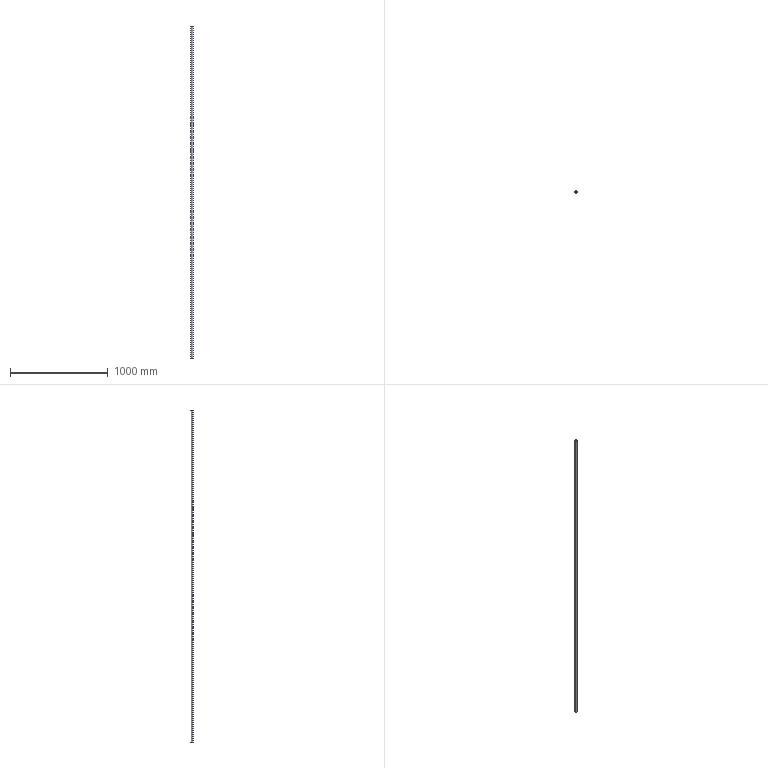Part | SolidWorks | features Extrusion 1 | 1 solid | 6 faces | box 25 x 25 x 3400 mm | volume 491345 mm3 | cylinder 4 | plane 2 | commonest cylinder face diameters 21 x2 25 x2
STEP:
#1=CARTESIAN_POINT('',(-10.5,0.,1700.));
#2=VERTEX_POINT('',#1);
#3=CARTESIAN_POINT('',(10.5,0.,1700.));
#4=VERTEX_POINT('',#3);
#5=CARTESIAN_POINT('',(0.,0.,1700.));
#6=DIRECTION('',(0.,0.,1.));
#7=DIRECTION('',(1.,0.,0.));
#8=AXIS2_PLACEMENT_3D('',#5,#6,#7);
#9=CIRCLE('',#8,10.5);
#10=EDGE_CURVE('',#2,#4,#9,.T.);
#11=ORIENTED_EDGE('',*,*,#10,.T.);
#12=CARTESIAN_POINT('',(10.5,0.,-1700.));
#13=VERTEX_POINT('',#12);
#14=CARTESIAN_POINT('',(10.5,0.,1700.));
#15=DIRECTION('',(0.,0.,-1.));
#16=VECTOR('',#15,1000.);
#17=LINE('',#14,#16);
#18=EDGE_CURVE('',#4,#13,#17,.T.);
#19=ORIENTED_EDGE('',*,*,#18,.T.);
#20=CARTESIAN_POINT('',(-10.5,0.,-1700.));
#21=VERTEX_POINT('',#20);
#22=CARTESIAN_POINT('',(0.,0.,-1700.));
#23=DIRECTION('',(0.,0.,1.));
#24=DIRECTION('',(1.,0.,0.));
#25=AXIS2_PLACEMENT_3D('',#22,#23,#24);
#26=CIRCLE('',#25,10.5);
#27=EDGE_CURVE('',#21,#13,#26,.T.);
#28=ORIENTED_EDGE('',*,*,#27,.F.);
#29=CARTESIAN_POINT('',(-10.5,0.,1700.));
#30=DIRECTION('',(0.,0.,-1.));
#31=VECTOR('',#30,1000.);
#32=LINE('',#29,#31);
#33=EDGE_CURVE('',#2,#21,#32,.T.);
#34=ORIENTED_EDGE('',*,*,#33,.F.);
#35=EDGE_LOOP('',(#11,#19,#28,#34));
#36=FACE_OUTER_BOUND('',#35,.T.);
#37=CARTESIAN_POINT('',(0.,0.,1700.));
#38=DIRECTION('',(0.,0.,-1.));
#39=DIRECTION('',(-1.,0.,0.));
#40=AXIS2_PLACEMENT_3D('',#37,#38,#39);
#41=CYLINDRICAL_SURFACE('',#40,10.5);
#42=ADVANCED_FACE('',(#36),#41,.F.);
#43=CARTESIAN_POINT('',(12.5,0.,1700.));
#44=VERTEX_POINT('',#43);
#45=CARTESIAN_POINT('',(-12.5,0.,1700.));
#46=VERTEX_POINT('',#45);
#47=CARTESIAN_POINT('',(0.,0.,1700.));
#48=DIRECTION('',(0.,0.,1.));
#49=DIRECTION('',(1.,0.,0.));
#50=AXIS2_PLACEMENT_3D('',#47,#48,#49);
#51=CIRCLE('',#50,12.5);
#52=EDGE_CURVE('',#44,#46,#51,.T.);
#53=ORIENTED_EDGE('',*,*,#52,.F.);
#54=CARTESIAN_POINT('',(12.5,0.,-1700.));
#55=VERTEX_POINT('',#54);
#56=CARTESIAN_POINT('',(12.5,0.,1700.));
#57=DIRECTION('',(0.,0.,-1.));
#58=VECTOR('',#57,1000.);
#59=LINE('',#56,#58);
#60=EDGE_CURVE('',#44,#55,#59,.T.);
#61=ORIENTED_EDGE('',*,*,#60,.T.);
#62=CARTESIAN_POINT('',(-12.5,0.,-1700.));
#63=VERTEX_POINT('',#62);
#64=CARTESIAN_POINT('',(0.,0.,-1700.));
#65=DIRECTION('',(0.,0.,1.));
#66=DIRECTION('',(1.,0.,0.));
#67=AXIS2_PLACEMENT_3D('',#64,#65,#66);
#68=CIRCLE('',#67,12.5);
#69=EDGE_CURVE('',#55,#63,#68,.T.);
#70=ORIENTED_EDGE('',*,*,#69,.T.);
#71=CARTESIAN_POINT('',(-12.5,0.,1700.));
#72=DIRECTION('',(0.,0.,-1.));
#73=VECTOR('',#72,1000.);
#74=LINE('',#71,#73);
#75=EDGE_CURVE('',#46,#63,#74,.T.);
#76=ORIENTED_EDGE('',*,*,#75,.F.);
#77=EDGE_LOOP('',(#53,#61,#70,#76));
#78=FACE_OUTER_BOUND('',#77,.T.);
#79=CARTESIAN_POINT('',(0.,0.,1700.));
#80=DIRECTION('',(0.,0.,-1.));
#81=DIRECTION('',(-1.,0.,0.));
#82=AXIS2_PLACEMENT_3D('',#79,#80,#81);
#83=CYLINDRICAL_SURFACE('',#82,12.5);
#84=ADVANCED_FACE('',(#78),#83,.T.);
#85=CARTESIAN_POINT('',(0.,0.,1700.));
#86=DIRECTION('',(0.,0.,1.));
#87=DIRECTION('',(1.,0.,0.));
#88=AXIS2_PLACEMENT_3D('',#85,#86,#87);
#89=CIRCLE('',#88,12.5);
#90=EDGE_CURVE('',#46,#44,#89,.T.);
#91=ORIENTED_EDGE('',*,*,#90,.T.);
#92=ORIENTED_EDGE('',*,*,#52,.T.);
#93=EDGE_LOOP('',(#91,#92));
#94=FACE_OUTER_BOUND('',#93,.T.);
#95=ORIENTED_EDGE('',*,*,#10,.F.);
#96=CARTESIAN_POINT('',(0.,0.,1700.));
#97=DIRECTION('',(0.,0.,1.));
#98=DIRECTION('',(1.,0.,0.));
#99=AXIS2_PLACEMENT_3D('',#96,#97,#98);
#100=CIRCLE('',#99,10.5);
#101=EDGE_CURVE('',#4,#2,#100,.T.);
#102=ORIENTED_EDGE('',*,*,#101,.F.);
#103=EDGE_LOOP('',(#95,#102));
#104=FACE_BOUND('',#103,.T.);
#105=CARTESIAN_POINT('',(0.,0.,1700.));
#106=DIRECTION('',(0.,0.,1.));
#107=DIRECTION('',(1.,0.,0.));
#108=AXIS2_PLACEMENT_3D('',#105,#106,#107);
#109=PLANE('',#108);
#110=ADVANCED_FACE('',(#94,#104),#109,.T.);
#111=CARTESIAN_POINT('',(0.,0.,-1700.));
#112=DIRECTION('',(0.,0.,1.));
#113=DIRECTION('',(1.,0.,0.));
#114=AXIS2_PLACEMENT_3D('',#111,#112,#113);
#115=CIRCLE('',#114,12.5);
#116=EDGE_CURVE('',#63,#55,#115,.T.);
#117=ORIENTED_EDGE('',*,*,#116,.F.);
#118=ORIENTED_EDGE('',*,*,#69,.F.);
#119=EDGE_LOOP('',(#117,#118));
#120=FACE_OUTER_BOUND('',#119,.T.);
#121=ORIENTED_EDGE('',*,*,#27,.T.);
#122=CARTESIAN_POINT('',(0.,0.,-1700.));
#123=DIRECTION('',(0.,0.,1.));
#124=DIRECTION('',(1.,0.,0.));
#125=AXIS2_PLACEMENT_3D('',#122,#123,#124);
#126=CIRCLE('',#125,10.5);
#127=EDGE_CURVE('',#13,#21,#126,.T.);
#128=ORIENTED_EDGE('',*,*,#127,.T.);
#129=EDGE_LOOP('',(#121,#128));
#130=FACE_BOUND('',#129,.T.);
#131=CARTESIAN_POINT('',(0.,0.,-1700.));
#132=DIRECTION('',(0.,0.,1.));
#133=DIRECTION('',(1.,0.,0.));
#134=AXIS2_PLACEMENT_3D('',#131,#132,#133);
#135=PLANE('',#134);
#136=ADVANCED_FACE('',(#120,#130),#135,.F.);
#137=ORIENTED_EDGE('',*,*,#60,.F.);
#138=ORIENTED_EDGE('',*,*,#90,.F.);
#139=ORIENTED_EDGE('',*,*,#75,.T.);
#140=ORIENTED_EDGE('',*,*,#116,.T.);
#141=EDGE_LOOP('',(#137,#138,#139,#140));
#142=FACE_OUTER_BOUND('',#141,.T.);
#143=CARTESIAN_POINT('',(0.,0.,1700.));
#144=DIRECTION('',(0.,0.,-1.));
#145=DIRECTION('',(-1.,0.,0.));
#146=AXIS2_PLACEMENT_3D('',#143,#144,#145);
#147=CYLINDRICAL_SURFACE('',#146,12.5);
#148=ADVANCED_FACE('',(#142),#147,.T.);
#149=ORIENTED_EDGE('',*,*,#18,.F.);
#150=ORIENTED_EDGE('',*,*,#101,.T.);
#151=ORIENTED_EDGE('',*,*,#33,.T.);
#152=ORIENTED_EDGE('',*,*,#127,.F.);
#153=EDGE_LOOP('',(#149,#150,#151,#152));
#154=FACE_OUTER_BOUND('',#153,.T.);
#155=CARTESIAN_POINT('',(0.,0.,1700.));
#156=DIRECTION('',(0.,0.,-1.));
#157=DIRECTION('',(-1.,0.,0.));
#158=AXIS2_PLACEMENT_3D('',#155,#156,#157);
#159=CYLINDRICAL_SURFACE('',#158,10.5);
#160=ADVANCED_FACE('',(#154),#159,.F.);
#161=CLOSED_SHELL('',(#42,#84,#110,#136,#148,#160));
#162=MANIFOLD_SOLID_BREP('',#161);
#163=CARTESIAN_POINT('',(0.,0.,0.));
#164=DIRECTION('',(0.,0.,1.));
#165=DIRECTION('',(1.,0.,0.));
#166=AXIS2_PLACEMENT_3D('',#163,#164,#165);
#167=(LENGTH_UNIT()NAMED_UNIT(*)SI_UNIT(.MILLI.,.METRE.));
#168=UNCERTAINTY_MEASURE_WITH_UNIT(LENGTH_MEASURE(0.00001),#167,'','');
#169=(NAMED_UNIT(*)PLANE_ANGLE_UNIT()SI_UNIT($,.RADIAN.));
#170=(NAMED_UNIT(*)SI_UNIT($,.STERADIAN.)SOLID_ANGLE_UNIT());
#171=(GEOMETRIC_REPRESENTATION_CONTEXT(3)GLOBAL_UNCERTAINTY_ASSIGNED_CONTEXT((#168))GLOBAL_UNIT_ASSIGNED_CONTEXT((#167,#169,#170))REPRESENTATION_CONTEXT('',''));
#172=ADVANCED_BREP_SHAPE_REPRESENTATION('',(#162,#166),#171);